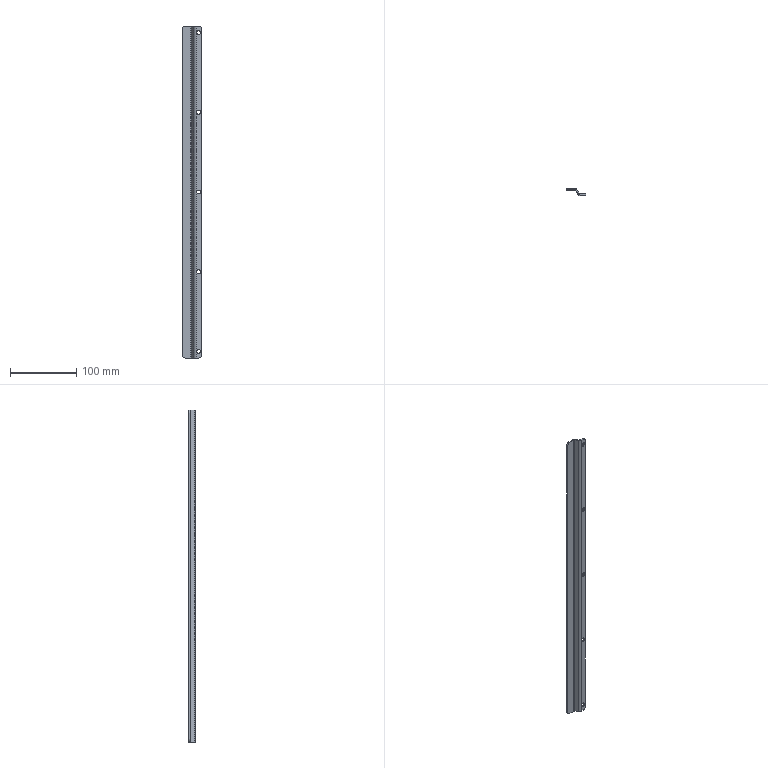Part | NX | features solid 2 | 1 solid | 28 faces | box 30 x 10 x 500 mm | volume 33531 mm3 | cylinder 18 | plane 10 | commonest cylinder face diameters 6 x10 10 x4 4 x2 8 x2
STEP:
#1=CARTESIAN_POINT('',(1918.,-650.,1125.));
#2=VERTEX_POINT('',#1);
#3=CARTESIAN_POINT('',(1918.,-648.,1125.));
#4=VERTEX_POINT('',#3);
#5=CARTESIAN_POINT('',(1918.,-1148.999,1125.));
#6=DIRECTION('',(0.,1.,0.));
#7=VECTOR('',#6,1000.);
#8=LINE('',#5,#7);
#9=EDGE_CURVE('',#2,#4,#8,.T.);
#10=ORIENTED_EDGE('',*,*,#9,.F.);
#11=CARTESIAN_POINT('',(1912.,-650.,1125.));
#12=VERTEX_POINT('',#11);
#13=CARTESIAN_POINT('',(1915.,-650.,1125.));
#14=DIRECTION('',(0.,1.,0.));
#15=DIRECTION('',(-1.,0.,0.));
#16=AXIS2_PLACEMENT_3D('',#13,#14,#15);
#17=CIRCLE('',#16,3.);
#18=EDGE_CURVE('',#12,#2,#17,.T.);
#19=ORIENTED_EDGE('',*,*,#18,.F.);
#20=CARTESIAN_POINT('',(1912.,-648.,1125.));
#21=VERTEX_POINT('',#20);
#22=CARTESIAN_POINT('',(1912.,-1148.999,1125.));
#23=DIRECTION('',(0.,1.,0.));
#24=VECTOR('',#23,1000.);
#25=LINE('',#22,#24);
#26=EDGE_CURVE('',#21,#12,#25,.F.);
#27=ORIENTED_EDGE('',*,*,#26,.F.);
#28=CARTESIAN_POINT('',(1915.,-648.,1125.));
#29=DIRECTION('',(0.,1.,0.));
#30=DIRECTION('',(0.,0.,-1.));
#31=AXIS2_PLACEMENT_3D('',#28,#29,#30);
#32=CIRCLE('',#31,3.);
#33=EDGE_CURVE('',#21,#4,#32,.T.);
#34=ORIENTED_EDGE('',*,*,#33,.T.);
#35=EDGE_LOOP('',(#10,#19,#27,#34));
#36=FACE_BOUND('',#35,.T.);
#37=CARTESIAN_POINT('',(1915.,-1148.999,1125.));
#38=DIRECTION('',(0.,1.,0.));
#39=DIRECTION('',(-1.,0.,0.));
#40=AXIS2_PLACEMENT_3D('',#37,#38,#39);
#41=CYLINDRICAL_SURFACE('',#40,3.);
#42=ADVANCED_FACE('',(#36),#41,.F.);
#43=CARTESIAN_POINT('',(1918.,-650.,645.));
#44=VERTEX_POINT('',#43);
#45=CARTESIAN_POINT('',(1918.,-648.,645.));
#46=VERTEX_POINT('',#45);
#47=CARTESIAN_POINT('',(1918.,-1148.999,645.));
#48=DIRECTION('',(0.,1.,0.));
#49=VECTOR('',#48,1000.);
#50=LINE('',#47,#49);
#51=EDGE_CURVE('',#44,#46,#50,.T.);
#52=ORIENTED_EDGE('',*,*,#51,.F.);
#53=CARTESIAN_POINT('',(1912.,-650.,645.));
#54=VERTEX_POINT('',#53);
#55=CARTESIAN_POINT('',(1915.,-650.,645.));
#56=DIRECTION('',(0.,1.,0.));
#57=DIRECTION('',(-1.,0.,0.));
#58=AXIS2_PLACEMENT_3D('',#55,#56,#57);
#59=CIRCLE('',#58,3.);
#60=EDGE_CURVE('',#54,#44,#59,.T.);
#61=ORIENTED_EDGE('',*,*,#60,.F.);
#62=CARTESIAN_POINT('',(1912.,-648.,645.));
#63=VERTEX_POINT('',#62);
#64=CARTESIAN_POINT('',(1912.,-1148.999,645.));
#65=DIRECTION('',(0.,1.,0.));
#66=VECTOR('',#65,1000.);
#67=LINE('',#64,#66);
#68=EDGE_CURVE('',#63,#54,#67,.F.);
#69=ORIENTED_EDGE('',*,*,#68,.F.);
#70=CARTESIAN_POINT('',(1915.,-648.,645.));
#71=DIRECTION('',(0.,1.,0.));
#72=DIRECTION('',(0.,0.,-1.));
#73=AXIS2_PLACEMENT_3D('',#70,#71,#72);
#74=CIRCLE('',#73,3.);
#75=EDGE_CURVE('',#63,#46,#74,.T.);
#76=ORIENTED_EDGE('',*,*,#75,.T.);
#77=EDGE_LOOP('',(#52,#61,#69,#76));
#78=FACE_BOUND('',#77,.T.);
#79=CARTESIAN_POINT('',(1915.,-1148.999,645.));
#80=DIRECTION('',(0.,1.,0.));
#81=DIRECTION('',(-1.,0.,0.));
#82=AXIS2_PLACEMENT_3D('',#79,#80,#81);
#83=CYLINDRICAL_SURFACE('',#82,3.);
#84=ADVANCED_FACE('',(#78),#83,.F.);
#85=CARTESIAN_POINT('',(1918.,-650.,1005.));
#86=VERTEX_POINT('',#85);
#87=CARTESIAN_POINT('',(1918.,-648.,1005.));
#88=VERTEX_POINT('',#87);
#89=CARTESIAN_POINT('',(1918.,-1148.999,1005.));
#90=DIRECTION('',(0.,1.,0.));
#91=VECTOR('',#90,1000.);
#92=LINE('',#89,#91);
#93=EDGE_CURVE('',#86,#88,#92,.T.);
#94=ORIENTED_EDGE('',*,*,#93,.F.);
#95=CARTESIAN_POINT('',(1912.,-650.,1005.));
#96=VERTEX_POINT('',#95);
#97=CARTESIAN_POINT('',(1915.,-650.,1005.));
#98=DIRECTION('',(0.,1.,0.));
#99=DIRECTION('',(-1.,0.,0.));
#100=AXIS2_PLACEMENT_3D('',#97,#98,#99);
#101=CIRCLE('',#100,3.);
#102=EDGE_CURVE('',#96,#86,#101,.T.);
#103=ORIENTED_EDGE('',*,*,#102,.F.);
#104=CARTESIAN_POINT('',(1912.,-648.,1005.));
#105=VERTEX_POINT('',#104);
#106=CARTESIAN_POINT('',(1912.,-1148.999,1005.));
#107=DIRECTION('',(0.,1.,0.));
#108=VECTOR('',#107,1000.);
#109=LINE('',#106,#108);
#110=EDGE_CURVE('',#105,#96,#109,.F.);
#111=ORIENTED_EDGE('',*,*,#110,.F.);
#112=CARTESIAN_POINT('',(1915.,-648.,1005.));
#113=DIRECTION('',(0.,1.,0.));
#114=DIRECTION('',(0.,0.,-1.));
#115=AXIS2_PLACEMENT_3D('',#112,#113,#114);
#116=CIRCLE('',#115,3.);
#117=EDGE_CURVE('',#105,#88,#116,.T.);
#118=ORIENTED_EDGE('',*,*,#117,.T.);
#119=EDGE_LOOP('',(#94,#103,#111,#118));
#120=FACE_BOUND('',#119,.T.);
#121=CARTESIAN_POINT('',(1915.,-1148.999,1005.));
#122=DIRECTION('',(0.,1.,0.));
#123=DIRECTION('',(-1.,0.,0.));
#124=AXIS2_PLACEMENT_3D('',#121,#122,#123);
#125=CYLINDRICAL_SURFACE('',#124,3.);
#126=ADVANCED_FACE('',(#120),#125,.F.);
#127=CARTESIAN_POINT('',(1918.,-648.,765.));
#128=VERTEX_POINT('',#127);
#129=CARTESIAN_POINT('',(1918.,-650.,765.));
#130=VERTEX_POINT('',#129);
#131=CARTESIAN_POINT('',(1918.,-1148.999,765.));
#132=DIRECTION('',(0.,1.,0.));
#133=VECTOR('',#132,1000.);
#134=LINE('',#131,#133);
#135=EDGE_CURVE('',#128,#130,#134,.F.);
#136=ORIENTED_EDGE('',*,*,#135,.T.);
#137=CARTESIAN_POINT('',(1912.,-650.,765.));
#138=VERTEX_POINT('',#137);
#139=CARTESIAN_POINT('',(1915.,-650.,765.));
#140=DIRECTION('',(0.,1.,0.));
#141=DIRECTION('',(-1.,0.,0.));
#142=AXIS2_PLACEMENT_3D('',#139,#140,#141);
#143=CIRCLE('',#142,3.);
#144=EDGE_CURVE('',#138,#130,#143,.T.);
#145=ORIENTED_EDGE('',*,*,#144,.F.);
#146=CARTESIAN_POINT('',(1912.,-648.,765.));
#147=VERTEX_POINT('',#146);
#148=CARTESIAN_POINT('',(1912.,-1148.999,765.));
#149=DIRECTION('',(0.,1.,0.));
#150=VECTOR('',#149,1000.);
#151=LINE('',#148,#150);
#152=EDGE_CURVE('',#138,#147,#151,.T.);
#153=ORIENTED_EDGE('',*,*,#152,.T.);
#154=CARTESIAN_POINT('',(1915.,-648.,765.));
#155=DIRECTION('',(0.,1.,0.));
#156=DIRECTION('',(0.,0.,-1.));
#157=AXIS2_PLACEMENT_3D('',#154,#155,#156);
#158=CIRCLE('',#157,3.);
#159=EDGE_CURVE('',#147,#128,#158,.T.);
#160=ORIENTED_EDGE('',*,*,#159,.T.);
#161=EDGE_LOOP('',(#136,#145,#153,#160));
#162=FACE_BOUND('',#161,.T.);
#163=CARTESIAN_POINT('',(1915.,-1148.999,765.));
#164=DIRECTION('',(0.,1.,0.));
#165=DIRECTION('',(-1.,0.,0.));
#166=AXIS2_PLACEMENT_3D('',#163,#164,#165);
#167=CYLINDRICAL_SURFACE('',#166,3.);
#168=ADVANCED_FACE('',(#162),#167,.F.);
#169=CARTESIAN_POINT('',(1918.,-650.,885.));
#170=VERTEX_POINT('',#169);
#171=CARTESIAN_POINT('',(1918.,-648.,885.));
#172=VERTEX_POINT('',#171);
#173=CARTESIAN_POINT('',(1918.,-1148.999,885.));
#174=DIRECTION('',(0.,1.,0.));
#175=VECTOR('',#174,1000.);
#176=LINE('',#173,#175);
#177=EDGE_CURVE('',#170,#172,#176,.T.);
#178=ORIENTED_EDGE('',*,*,#177,.F.);
#179=CARTESIAN_POINT('',(1912.,-650.,885.));
#180=VERTEX_POINT('',#179);
#181=CARTESIAN_POINT('',(1915.,-650.,885.));
#182=DIRECTION('',(0.,1.,0.));
#183=DIRECTION('',(-1.,0.,0.));
#184=AXIS2_PLACEMENT_3D('',#181,#182,#183);
#185=CIRCLE('',#184,3.);
#186=EDGE_CURVE('',#180,#170,#185,.T.);
#187=ORIENTED_EDGE('',*,*,#186,.F.);
#188=CARTESIAN_POINT('',(1912.,-648.,885.));
#189=VERTEX_POINT('',#188);
#190=CARTESIAN_POINT('',(1912.,-1148.999,885.));
#191=DIRECTION('',(0.,1.,0.));
#192=VECTOR('',#191,1000.);
#193=LINE('',#190,#192);
#194=EDGE_CURVE('',#189,#180,#193,.F.);
#195=ORIENTED_EDGE('',*,*,#194,.F.);
#196=CARTESIAN_POINT('',(1915.,-648.,885.));
#197=DIRECTION('',(0.,1.,0.));
#198=DIRECTION('',(0.,0.,-1.));
#199=AXIS2_PLACEMENT_3D('',#196,#197,#198);
#200=CIRCLE('',#199,3.);
#201=EDGE_CURVE('',#189,#172,#200,.T.);
#202=ORIENTED_EDGE('',*,*,#201,.T.);
#203=EDGE_LOOP('',(#178,#187,#195,#202));
#204=FACE_BOUND('',#203,.T.);
#205=CARTESIAN_POINT('',(1915.,-1148.999,885.));
#206=DIRECTION('',(0.,1.,0.));
#207=DIRECTION('',(-1.,0.,0.));
#208=AXIS2_PLACEMENT_3D('',#205,#206,#207);
#209=CYLINDRICAL_SURFACE('',#208,3.);
#210=ADVANCED_FACE('',(#204),#209,.F.);
#211=CARTESIAN_POINT('',(1895.,-642.,1135.));
#212=VERTEX_POINT('',#211);
#213=CARTESIAN_POINT('',(1890.,-642.,1130.));
#214=VERTEX_POINT('',#213);
#215=CARTESIAN_POINT('',(1895.,-642.,1130.));
#216=DIRECTION('',(0.,-1.,0.));
#217=DIRECTION('',(0.,0.,1.));
#218=AXIS2_PLACEMENT_3D('',#215,#216,#217);
#219=CIRCLE('',#218,5.);
#220=EDGE_CURVE('',#212,#214,#219,.T.);
#221=ORIENTED_EDGE('',*,*,#220,.F.);
#222=CARTESIAN_POINT('',(1895.,-640.,1135.));
#223=VERTEX_POINT('',#222);
#224=CARTESIAN_POINT('',(1895.,-648.,1135.));
#225=DIRECTION('',(0.,-1.,0.));
#226=VECTOR('',#225,1000.);
#227=LINE('',#224,#226);
#228=EDGE_CURVE('',#223,#212,#227,.T.);
#229=ORIENTED_EDGE('',*,*,#228,.F.);
#230=CARTESIAN_POINT('',(1890.,-640.,1130.));
#231=VERTEX_POINT('',#230);
#232=CARTESIAN_POINT('',(1895.,-640.,1130.));
#233=DIRECTION('',(0.,1.,0.));
#234=DIRECTION('',(0.,0.,1.));
#235=AXIS2_PLACEMENT_3D('',#232,#233,#234);
#236=CIRCLE('',#235,5.);
#237=EDGE_CURVE('',#231,#223,#236,.T.);
#238=ORIENTED_EDGE('',*,*,#237,.F.);
#239=CARTESIAN_POINT('',(1890.,-640.,1130.));
#240=DIRECTION('',(0.,1.,0.));
#241=VECTOR('',#240,1000.);
#242=LINE('',#239,#241);
#243=EDGE_CURVE('',#214,#231,#242,.T.);
#244=ORIENTED_EDGE('',*,*,#243,.F.);
#245=EDGE_LOOP('',(#221,#229,#238,#244));
#246=FACE_BOUND('',#245,.T.);
#247=CARTESIAN_POINT('',(1895.,-640.,1130.));
#248=DIRECTION('',(0.,-1.,0.));
#249=DIRECTION('',(0.,0.,-1.));
#250=AXIS2_PLACEMENT_3D('',#247,#248,#249);
#251=CYLINDRICAL_SURFACE('',#250,5.);
#252=ADVANCED_FACE('',(#246),#251,.T.);
#253=CARTESIAN_POINT('',(1920.,-650.,1130.));
#254=VERTEX_POINT('',#253);
#255=CARTESIAN_POINT('',(1915.,-650.,1135.));
#256=VERTEX_POINT('',#255);
#257=CARTESIAN_POINT('',(1915.,-650.,1130.));
#258=DIRECTION('',(0.,-1.,0.));
#259=DIRECTION('',(-1.,0.,0.));
#260=AXIS2_PLACEMENT_3D('',#257,#258,#259);
#261=CIRCLE('',#260,5.);
#262=EDGE_CURVE('',#254,#256,#261,.T.);
#263=ORIENTED_EDGE('',*,*,#262,.F.);
#264=CARTESIAN_POINT('',(1920.,-648.,1130.));
#265=VERTEX_POINT('',#264);
#266=CARTESIAN_POINT('',(1920.,-648.,1130.));
#267=DIRECTION('',(0.,-1.,0.));
#268=VECTOR('',#267,1000.);
#269=LINE('',#266,#268);
#270=EDGE_CURVE('',#265,#254,#269,.T.);
#271=ORIENTED_EDGE('',*,*,#270,.F.);
#272=CARTESIAN_POINT('',(1915.,-648.,1135.));
#273=VERTEX_POINT('',#272);
#274=CARTESIAN_POINT('',(1915.,-648.,1130.));
#275=DIRECTION('',(0.,1.,0.));
#276=DIRECTION('',(-1.,0.,0.));
#277=AXIS2_PLACEMENT_3D('',#274,#275,#276);
#278=CIRCLE('',#277,5.);
#279=EDGE_CURVE('',#273,#265,#278,.T.);
#280=ORIENTED_EDGE('',*,*,#279,.F.);
#281=CARTESIAN_POINT('',(1915.,-648.,1135.));
#282=DIRECTION('',(0.,1.,0.));
#283=VECTOR('',#282,1000.);
#284=LINE('',#281,#283);
#285=EDGE_CURVE('',#256,#273,#284,.T.);
#286=ORIENTED_EDGE('',*,*,#285,.F.);
#287=EDGE_LOOP('',(#263,#271,#280,#286));
#288=FACE_BOUND('',#287,.T.);
#289=CARTESIAN_POINT('',(1915.,-648.,1130.));
#290=DIRECTION('',(0.,1.,0.));
#291=DIRECTION('',(-1.,0.,0.));
#292=AXIS2_PLACEMENT_3D('',#289,#290,#291);
#293=CYLINDRICAL_SURFACE('',#292,5.);
#294=ADVANCED_FACE('',(#288),#293,.T.);
#295=CARTESIAN_POINT('',(1890.,-642.,640.));
#296=VERTEX_POINT('',#295);
#297=CARTESIAN_POINT('',(1895.,-642.,635.));
#298=VERTEX_POINT('',#297);
#299=CARTESIAN_POINT('',(1895.,-642.,640.));
#300=DIRECTION('',(0.,-1.,0.));
#301=DIRECTION('',(0.,0.,1.));
#302=AXIS2_PLACEMENT_3D('',#299,#300,#301);
#303=CIRCLE('',#302,5.);
#304=EDGE_CURVE('',#296,#298,#303,.T.);
#305=ORIENTED_EDGE('',*,*,#304,.F.);
#306=CARTESIAN_POINT('',(1890.,-640.,640.));
#307=VERTEX_POINT('',#306);
#308=CARTESIAN_POINT('',(1890.,-640.,640.));
#309=DIRECTION('',(0.,-1.,0.));
#310=VECTOR('',#309,1000.);
#311=LINE('',#308,#310);
#312=EDGE_CURVE('',#307,#296,#311,.T.);
#313=ORIENTED_EDGE('',*,*,#312,.F.);
#314=CARTESIAN_POINT('',(1895.,-640.,635.));
#315=VERTEX_POINT('',#314);
#316=CARTESIAN_POINT('',(1895.,-640.,640.));
#317=DIRECTION('',(0.,1.,0.));
#318=DIRECTION('',(0.,0.,1.));
#319=AXIS2_PLACEMENT_3D('',#316,#317,#318);
#320=CIRCLE('',#319,5.);
#321=EDGE_CURVE('',#315,#307,#320,.T.);
#322=ORIENTED_EDGE('',*,*,#321,.F.);
#323=CARTESIAN_POINT('',(1895.,-640.,635.));
#324=DIRECTION('',(0.,1.,0.));
#325=VECTOR('',#324,1000.);
#326=LINE('',#323,#325);
#327=EDGE_CURVE('',#298,#315,#326,.T.);
#328=ORIENTED_EDGE('',*,*,#327,.F.);
#329=EDGE_LOOP('',(#305,#313,#322,#328));
#330=FACE_BOUND('',#329,.T.);
#331=CARTESIAN_POINT('',(1895.,-640.,640.));
#332=DIRECTION('',(0.,1.,0.));
#333=DIRECTION('',(0.,0.,1.));
#334=AXIS2_PLACEMENT_3D('',#331,#332,#333);
#335=CYLINDRICAL_SURFACE('',#334,5.);
#336=ADVANCED_FACE('',(#330),#335,.T.);
#337=CARTESIAN_POINT('',(1915.,-650.,635.));
#338=VERTEX_POINT('',#337);
#339=CARTESIAN_POINT('',(1920.,-650.,640.));
#340=VERTEX_POINT('',#339);
#341=CARTESIAN_POINT('',(1915.,-650.,640.));
#342=DIRECTION('',(0.,-1.,0.));
#343=DIRECTION('',(-1.,0.,0.));
#344=AXIS2_PLACEMENT_3D('',#341,#342,#343);
#345=CIRCLE('',#344,5.);
#346=EDGE_CURVE('',#338,#340,#345,.T.);
#347=ORIENTED_EDGE('',*,*,#346,.F.);
#348=CARTESIAN_POINT('',(1915.,-648.,635.));
#349=VERTEX_POINT('',#348);
#350=CARTESIAN_POINT('',(1915.,-640.,635.));
#351=DIRECTION('',(0.,-1.,0.));
#352=VECTOR('',#351,1000.);
#353=LINE('',#350,#352);
#354=EDGE_CURVE('',#349,#338,#353,.T.);
#355=ORIENTED_EDGE('',*,*,#354,.F.);
#356=CARTESIAN_POINT('',(1920.,-648.,640.));
#357=VERTEX_POINT('',#356);
#358=CARTESIAN_POINT('',(1915.,-648.,640.));
#359=DIRECTION('',(0.,1.,0.));
#360=DIRECTION('',(-1.,0.,0.));
#361=AXIS2_PLACEMENT_3D('',#358,#359,#360);
#362=CIRCLE('',#361,5.);
#363=EDGE_CURVE('',#357,#349,#362,.T.);
#364=ORIENTED_EDGE('',*,*,#363,.F.);
#365=CARTESIAN_POINT('',(1920.,-648.,640.));
#366=DIRECTION('',(0.,1.,0.));
#367=VECTOR('',#366,1000.);
#368=LINE('',#365,#367);
#369=EDGE_CURVE('',#340,#357,#368,.T.);
#370=ORIENTED_EDGE('',*,*,#369,.F.);
#371=EDGE_LOOP('',(#347,#355,#364,#370));
#372=FACE_BOUND('',#371,.T.);
#373=CARTESIAN_POINT('',(1915.,-648.,640.));
#374=DIRECTION('',(0.,-1.,0.));
#375=DIRECTION('',(1.,0.,0.));
#376=AXIS2_PLACEMENT_3D('',#373,#374,#375);
#377=CYLINDRICAL_SURFACE('',#376,5.);
#378=ADVANCED_FACE('',(#372),#377,.T.);
#379=CARTESIAN_POINT('',(1890.,-642.,635.));
#380=DIRECTION('',(0.,0.,1.));
#381=VECTOR('',#380,1000.);
#382=LINE('',#379,#381);
#383=EDGE_CURVE('',#296,#214,#382,.T.);
#384=ORIENTED_EDGE('',*,*,#383,.F.);
#385=ORIENTED_EDGE('',*,*,#304,.T.);
#386=CARTESIAN_POINT('',(1902.783,-642.,635.));
#387=VERTEX_POINT('',#386);
#388=CARTESIAN_POINT('',(1905.,-642.,635.));
#389=DIRECTION('',(-1.,0.,0.));
#390=VECTOR('',#389,1000.);
#391=LINE('',#388,#390);
#392=EDGE_CURVE('',#387,#298,#391,.T.);
#393=ORIENTED_EDGE('',*,*,#392,.F.);
#394=CARTESIAN_POINT('',(1902.783,-642.,1135.));
#395=VERTEX_POINT('',#394);
#396=CARTESIAN_POINT('',(1902.783,-642.,635.));
#397=DIRECTION('',(0.,0.,1.));
#398=VECTOR('',#397,1000.);
#399=LINE('',#396,#398);
#400=EDGE_CURVE('',#387,#395,#399,.T.);
#401=ORIENTED_EDGE('',*,*,#400,.T.);
#402=CARTESIAN_POINT('',(1905.,-642.,1135.));
#403=DIRECTION('',(-1.,0.,0.));
#404=VECTOR('',#403,1000.);
#405=LINE('',#402,#404);
#406=EDGE_CURVE('',#395,#212,#405,.T.);
#407=ORIENTED_EDGE('',*,*,#406,.T.);
#408=ORIENTED_EDGE('',*,*,#220,.T.);
#409=EDGE_LOOP('',(#384,#385,#393,#401,#407,#408));
#410=FACE_BOUND('',#409,.T.);
#411=CARTESIAN_POINT('',(1905.,-642.,635.));
#412=DIRECTION('',(0.,1.,0.));
#413=DIRECTION('',(0.,0.,-1.));
#414=AXIS2_PLACEMENT_3D('',#411,#412,#413);
#415=PLANE('',#414);
#416=ADVANCED_FACE('',(#410),#415,.F.);
#417=CARTESIAN_POINT('',(1904.479,-642.94,1135.));
#418=VERTEX_POINT('',#417);
#419=CARTESIAN_POINT('',(1902.783,-644.,1135.));
#420=DIRECTION('',(0.,0.,1.));
#421=DIRECTION('',(0.,-1.,0.));
#422=AXIS2_PLACEMENT_3D('',#419,#420,#421);
#423=CIRCLE('',#422,2.);
#424=EDGE_CURVE('',#418,#395,#423,.T.);
#425=ORIENTED_EDGE('',*,*,#424,.T.);
#426=ORIENTED_EDGE('',*,*,#400,.F.);
#427=CARTESIAN_POINT('',(1904.479,-642.94,635.));
#428=VERTEX_POINT('',#427);
#429=CARTESIAN_POINT('',(1902.783,-644.,635.));
#430=DIRECTION('',(0.,0.,1.));
#431=DIRECTION('',(0.,-1.,0.));
#432=AXIS2_PLACEMENT_3D('',#429,#430,#431);
#433=CIRCLE('',#432,2.);
#434=EDGE_CURVE('',#428,#387,#433,.T.);
#435=ORIENTED_EDGE('',*,*,#434,.F.);
#436=CARTESIAN_POINT('',(1904.479,-642.94,635.));
#437=DIRECTION('',(0.,0.,1.));
#438=VECTOR('',#437,1000.);
#439=LINE('',#436,#438);
#440=EDGE_CURVE('',#428,#418,#439,.T.);
#441=ORIENTED_EDGE('',*,*,#440,.T.);
#442=EDGE_LOOP('',(#425,#426,#435,#441));
#443=FACE_BOUND('',#442,.T.);
#444=CARTESIAN_POINT('',(1902.783,-644.,635.));
#445=DIRECTION('',(0.,0.,1.));
#446=DIRECTION('',(0.,-1.,0.));
#447=AXIS2_PLACEMENT_3D('',#444,#445,#446);
#448=CYLINDRICAL_SURFACE('',#447,2.);
#449=ADVANCED_FACE('',(#443),#448,.F.);
#450=CARTESIAN_POINT('',(1907.717,-648.12,1135.));
#451=VERTEX_POINT('',#450);
#452=CARTESIAN_POINT('',(1908.304,-649.06,1135.));
#453=DIRECTION('',(-0.53,0.848,0.));
#454=VECTOR('',#453,1000.);
#455=LINE('',#452,#454);
#456=EDGE_CURVE('',#451,#418,#455,.T.);
#457=ORIENTED_EDGE('',*,*,#456,.T.);
#458=ORIENTED_EDGE('',*,*,#440,.F.);
#459=CARTESIAN_POINT('',(1907.717,-648.12,635.));
#460=VERTEX_POINT('',#459);
#461=CARTESIAN_POINT('',(1908.304,-649.06,635.));
#462=DIRECTION('',(-0.53,0.848,0.));
#463=VECTOR('',#462,1000.);
#464=LINE('',#461,#463);
#465=EDGE_CURVE('',#460,#428,#464,.T.);
#466=ORIENTED_EDGE('',*,*,#465,.F.);
#467=CARTESIAN_POINT('',(1907.717,-648.12,635.));
#468=DIRECTION('',(0.,0.,1.));
#469=VECTOR('',#468,1000.);
#470=LINE('',#467,#469);
#471=EDGE_CURVE('',#460,#451,#470,.T.);
#472=ORIENTED_EDGE('',*,*,#471,.T.);
#473=EDGE_LOOP('',(#457,#458,#466,#472));
#474=FACE_BOUND('',#473,.T.);
#475=CARTESIAN_POINT('',(1908.304,-649.06,635.));
#476=DIRECTION('',(0.848,0.53,0.));
#477=DIRECTION('',(0.,0.,-1.));
#478=AXIS2_PLACEMENT_3D('',#475,#476,#477);
#479=PLANE('',#478);
#480=ADVANCED_FACE('',(#474),#479,.F.);
#481=CARTESIAN_POINT('',(1911.108,-650.,1135.));
#482=VERTEX_POINT('',#481);
#483=CARTESIAN_POINT('',(1911.108,-646.,1135.));
#484=DIRECTION('',(0.,0.,-1.));
#485=DIRECTION('',(0.,-1.,0.));
#486=AXIS2_PLACEMENT_3D('',#483,#484,#485);
#487=CIRCLE('',#486,4.);
#488=EDGE_CURVE('',#482,#451,#487,.T.);
#489=ORIENTED_EDGE('',*,*,#488,.T.);
#490=ORIENTED_EDGE('',*,*,#471,.F.);
#491=CARTESIAN_POINT('',(1911.108,-650.,635.));
#492=VERTEX_POINT('',#491);
#493=CARTESIAN_POINT('',(1911.108,-646.,635.));
#494=DIRECTION('',(0.,0.,-1.));
#495=DIRECTION('',(0.,-1.,0.));
#496=AXIS2_PLACEMENT_3D('',#493,#494,#495);
#497=CIRCLE('',#496,4.);
#498=EDGE_CURVE('',#492,#460,#497,.T.);
#499=ORIENTED_EDGE('',*,*,#498,.F.);
#500=CARTESIAN_POINT('',(1911.108,-650.,635.));
#501=DIRECTION('',(0.,0.,1.));
#502=VECTOR('',#501,1000.);
#503=LINE('',#500,#502);
#504=EDGE_CURVE('',#492,#482,#503,.T.);
#505=ORIENTED_EDGE('',*,*,#504,.T.);
#506=EDGE_LOOP('',(#489,#490,#499,#505));
#507=FACE_BOUND('',#506,.T.);
#508=CARTESIAN_POINT('',(1911.108,-646.,635.));
#509=DIRECTION('',(0.,0.,1.));
#510=DIRECTION('',(0.,-1.,0.));
#511=AXIS2_PLACEMENT_3D('',#508,#509,#510);
#512=CYLINDRICAL_SURFACE('',#511,4.);
#513=ADVANCED_FACE('',(#507),#512,.T.);
#514=ORIENTED_EDGE('',*,*,#186,.T.);
#515=CARTESIAN_POINT('',(1915.,-650.,885.));
#516=DIRECTION('',(0.,1.,0.));
#517=DIRECTION('',(-1.,0.,0.));
#518=AXIS2_PLACEMENT_3D('',#515,#516,#517);
#519=CIRCLE('',#518,3.);
#520=EDGE_CURVE('',#170,#180,#519,.T.);
#521=ORIENTED_EDGE('',*,*,#520,.T.);
#522=EDGE_LOOP('',(#514,#521));
#523=FACE_BOUND('',#522,.T.);
#524=ORIENTED_EDGE('',*,*,#144,.T.);
#525=CARTESIAN_POINT('',(1915.,-650.,765.));
#526=DIRECTION('',(0.,1.,0.));
#527=DIRECTION('',(-1.,0.,0.));
#528=AXIS2_PLACEMENT_3D('',#525,#526,#527);
#529=CIRCLE('',#528,3.);
#530=EDGE_CURVE('',#130,#138,#529,.T.);
#531=ORIENTED_EDGE('',*,*,#530,.T.);
#532=EDGE_LOOP('',(#524,#531));
#533=FACE_BOUND('',#532,.T.);
#534=ORIENTED_EDGE('',*,*,#102,.T.);
#535=CARTESIAN_POINT('',(1915.,-650.,1005.));
#536=DIRECTION('',(0.,1.,0.));
#537=DIRECTION('',(-1.,0.,0.));
#538=AXIS2_PLACEMENT_3D('',#535,#536,#537);
#539=CIRCLE('',#538,3.);
#540=EDGE_CURVE('',#86,#96,#539,.T.);
#541=ORIENTED_EDGE('',*,*,#540,.T.);
#542=EDGE_LOOP('',(#534,#541));
#543=FACE_BOUND('',#542,.T.);
#544=ORIENTED_EDGE('',*,*,#60,.T.);
#545=CARTESIAN_POINT('',(1915.,-650.,645.));
#546=DIRECTION('',(0.,1.,0.));
#547=DIRECTION('',(-1.,0.,0.));
#548=AXIS2_PLACEMENT_3D('',#545,#546,#547);
#549=CIRCLE('',#548,3.);
#550=EDGE_CURVE('',#44,#54,#549,.T.);
#551=ORIENTED_EDGE('',*,*,#550,.T.);
#552=EDGE_LOOP('',(#544,#551));
#553=FACE_BOUND('',#552,.T.);
#554=ORIENTED_EDGE('',*,*,#18,.T.);
#555=CARTESIAN_POINT('',(1915.,-650.,1125.));
#556=DIRECTION('',(0.,1.,0.));
#557=DIRECTION('',(-1.,0.,0.));
#558=AXIS2_PLACEMENT_3D('',#555,#556,#557);
#559=CIRCLE('',#558,3.);
#560=EDGE_CURVE('',#2,#12,#559,.T.);
#561=ORIENTED_EDGE('',*,*,#560,.T.);
#562=EDGE_LOOP('',(#554,#561));
#563=FACE_BOUND('',#562,.T.);
#564=CARTESIAN_POINT('',(1920.,-650.,635.));
#565=DIRECTION('',(-1.,0.,0.));
#566=VECTOR('',#565,1000.);
#567=LINE('',#564,#566);
#568=EDGE_CURVE('',#338,#492,#567,.T.);
#569=ORIENTED_EDGE('',*,*,#568,.F.);
#570=ORIENTED_EDGE('',*,*,#346,.T.);
#571=CARTESIAN_POINT('',(1920.,-650.,635.));
#572=DIRECTION('',(0.,0.,1.));
#573=VECTOR('',#572,1000.);
#574=LINE('',#571,#573);
#575=EDGE_CURVE('',#340,#254,#574,.T.);
#576=ORIENTED_EDGE('',*,*,#575,.T.);
#577=ORIENTED_EDGE('',*,*,#262,.T.);
#578=CARTESIAN_POINT('',(1920.,-650.,1135.));
#579=DIRECTION('',(-1.,0.,0.));
#580=VECTOR('',#579,1000.);
#581=LINE('',#578,#580);
#582=EDGE_CURVE('',#256,#482,#581,.T.);
#583=ORIENTED_EDGE('',*,*,#582,.T.);
#584=ORIENTED_EDGE('',*,*,#504,.F.);
#585=EDGE_LOOP('',(#569,#570,#576,#577,#583,#584));
#586=FACE_BOUND('',#585,.T.);
#587=CARTESIAN_POINT('',(1920.,-650.,635.));
#588=DIRECTION('',(0.,1.,0.));
#589=DIRECTION('',(0.,0.,-1.));
#590=AXIS2_PLACEMENT_3D('',#587,#588,#589);
#591=PLANE('',#590);
#592=ADVANCED_FACE('',(#523,#533,#543,#553,#563,#586),#591,.F.);
#593=CARTESIAN_POINT('',(1902.783,-640.,635.));
#594=VERTEX_POINT('',#593);
#595=CARTESIAN_POINT('',(1905.,-640.,635.));
#596=DIRECTION('',(-1.,0.,0.));
#597=VECTOR('',#596,1000.);
#598=LINE('',#595,#597);
#599=EDGE_CURVE('',#594,#315,#598,.T.);
#600=ORIENTED_EDGE('',*,*,#599,.T.);
#601=ORIENTED_EDGE('',*,*,#321,.T.);
#602=CARTESIAN_POINT('',(1890.,-640.,635.));
#603=DIRECTION('',(0.,0.,1.));
#604=VECTOR('',#603,1000.);
#605=LINE('',#602,#604);
#606=EDGE_CURVE('',#307,#231,#605,.T.);
#607=ORIENTED_EDGE('',*,*,#606,.T.);
#608=ORIENTED_EDGE('',*,*,#237,.T.);
#609=CARTESIAN_POINT('',(1902.783,-640.,1135.));
#610=VERTEX_POINT('',#609);
#611=CARTESIAN_POINT('',(1905.,-640.,1135.));
#612=DIRECTION('',(-1.,0.,0.));
#613=VECTOR('',#612,1000.);
#614=LINE('',#611,#613);
#615=EDGE_CURVE('',#610,#223,#614,.T.);
#616=ORIENTED_EDGE('',*,*,#615,.F.);
#617=CARTESIAN_POINT('',(1902.783,-640.,635.));
#618=DIRECTION('',(0.,0.,1.));
#619=VECTOR('',#618,1000.);
#620=LINE('',#617,#619);
#621=EDGE_CURVE('',#594,#610,#620,.T.);
#622=ORIENTED_EDGE('',*,*,#621,.F.);
#623=EDGE_LOOP('',(#600,#601,#607,#608,#616,#622));
#624=FACE_BOUND('',#623,.T.);
#625=CARTESIAN_POINT('',(1905.,-640.,635.));
#626=DIRECTION('',(0.,1.,0.));
#627=DIRECTION('',(0.,0.,-1.));
#628=AXIS2_PLACEMENT_3D('',#625,#626,#627);
#629=PLANE('',#628);
#630=ADVANCED_FACE('',(#624),#629,.T.);
#631=CARTESIAN_POINT('',(1906.175,-641.88,1135.));
#632=VERTEX_POINT('',#631);
#633=CARTESIAN_POINT('',(1902.783,-644.,1135.));
#634=DIRECTION('',(0.,0.,1.));
#635=DIRECTION('',(0.,1.,0.));
#636=AXIS2_PLACEMENT_3D('',#633,#634,#635);
#637=CIRCLE('',#636,4.);
#638=EDGE_CURVE('',#632,#610,#637,.T.);
#639=ORIENTED_EDGE('',*,*,#638,.F.);
#640=CARTESIAN_POINT('',(1906.175,-641.88,635.));
#641=VERTEX_POINT('',#640);
#642=CARTESIAN_POINT('',(1906.175,-641.88,635.));
#643=DIRECTION('',(0.,0.,1.));
#644=VECTOR('',#643,1000.);
#645=LINE('',#642,#644);
#646=EDGE_CURVE('',#641,#632,#645,.T.);
#647=ORIENTED_EDGE('',*,*,#646,.F.);
#648=CARTESIAN_POINT('',(1902.783,-644.,635.));
#649=DIRECTION('',(0.,0.,1.));
#650=DIRECTION('',(0.,1.,0.));
#651=AXIS2_PLACEMENT_3D('',#648,#649,#650);
#652=CIRCLE('',#651,4.);
#653=EDGE_CURVE('',#641,#594,#652,.T.);
#654=ORIENTED_EDGE('',*,*,#653,.T.);
#655=ORIENTED_EDGE('',*,*,#621,.T.);
#656=EDGE_LOOP('',(#639,#647,#654,#655));
#657=FACE_BOUND('',#656,.T.);
#658=CARTESIAN_POINT('',(1902.783,-644.,635.));
#659=DIRECTION('',(0.,0.,1.));
#660=DIRECTION('',(0.,-1.,0.));
#661=AXIS2_PLACEMENT_3D('',#658,#659,#660);
#662=CYLINDRICAL_SURFACE('',#661,4.);
#663=ADVANCED_FACE('',(#657),#662,.T.);
#664=CARTESIAN_POINT('',(1909.412,-647.06,1135.));
#665=VERTEX_POINT('',#664);
#666=CARTESIAN_POINT('',(1910.,-648.,1135.));
#667=DIRECTION('',(-0.53,0.848,0.));
#668=VECTOR('',#667,1000.);
#669=LINE('',#666,#668);
#670=EDGE_CURVE('',#665,#632,#669,.T.);
#671=ORIENTED_EDGE('',*,*,#670,.F.);
#672=CARTESIAN_POINT('',(1909.412,-647.06,635.));
#673=VERTEX_POINT('',#672);
#674=CARTESIAN_POINT('',(1909.412,-647.06,635.));
#675=DIRECTION('',(0.,0.,1.));
#676=VECTOR('',#675,1000.);
#677=LINE('',#674,#676);
#678=EDGE_CURVE('',#673,#665,#677,.T.);
#679=ORIENTED_EDGE('',*,*,#678,.F.);
#680=CARTESIAN_POINT('',(1910.,-648.,635.));
#681=DIRECTION('',(-0.53,0.848,0.));
#682=VECTOR('',#681,1000.);
#683=LINE('',#680,#682);
#684=EDGE_CURVE('',#673,#641,#683,.T.);
#685=ORIENTED_EDGE('',*,*,#684,.T.);
#686=ORIENTED_EDGE('',*,*,#646,.T.);
#687=EDGE_LOOP('',(#671,#679,#685,#686));
#688=FACE_BOUND('',#687,.T.);
#689=CARTESIAN_POINT('',(1910.,-648.,635.));
#690=DIRECTION('',(0.848,0.53,0.));
#691=DIRECTION('',(0.,0.,-1.));
#692=AXIS2_PLACEMENT_3D('',#689,#690,#691);
#693=PLANE('',#692);
#694=ADVANCED_FACE('',(#688),#693,.T.);
#695=CARTESIAN_POINT('',(1911.108,-648.,1135.));
#696=VERTEX_POINT('',#695);
#697=CARTESIAN_POINT('',(1911.108,-646.,1135.));
#698=DIRECTION('',(0.,0.,-1.));
#699=DIRECTION('',(0.,-1.,0.));
#700=AXIS2_PLACEMENT_3D('',#697,#698,#699);
#701=CIRCLE('',#700,2.);
#702=EDGE_CURVE('',#696,#665,#701,.T.);
#703=ORIENTED_EDGE('',*,*,#702,.F.);
#704=CARTESIAN_POINT('',(1911.108,-648.,635.));
#705=VERTEX_POINT('',#704);
#706=CARTESIAN_POINT('',(1911.108,-648.,635.));
#707=DIRECTION('',(0.,0.,1.));
#708=VECTOR('',#707,1000.);
#709=LINE('',#706,#708);
#710=EDGE_CURVE('',#705,#696,#709,.T.);
#711=ORIENTED_EDGE('',*,*,#710,.F.);
#712=CARTESIAN_POINT('',(1911.108,-646.,635.));
#713=DIRECTION('',(0.,0.,-1.));
#714=DIRECTION('',(0.,-1.,0.));
#715=AXIS2_PLACEMENT_3D('',#712,#713,#714);
#716=CIRCLE('',#715,2.);
#717=EDGE_CURVE('',#705,#673,#716,.T.);
#718=ORIENTED_EDGE('',*,*,#717,.T.);
#719=ORIENTED_EDGE('',*,*,#678,.T.);
#720=EDGE_LOOP('',(#703,#711,#718,#719));
#721=FACE_BOUND('',#720,.T.);
#722=CARTESIAN_POINT('',(1911.108,-646.,635.));
#723=DIRECTION('',(0.,0.,1.));
#724=DIRECTION('',(0.,-1.,0.));
#725=AXIS2_PLACEMENT_3D('',#722,#723,#724);
#726=CYLINDRICAL_SURFACE('',#725,2.);
#727=ADVANCED_FACE('',(#721),#726,.F.);
#728=ORIENTED_EDGE('',*,*,#201,.F.);
#729=CARTESIAN_POINT('',(1915.,-648.,885.));
#730=DIRECTION('',(0.,1.,0.));
#731=DIRECTION('',(0.,0.,-1.));
#732=AXIS2_PLACEMENT_3D('',#729,#730,#731);
#733=CIRCLE('',#732,3.);
#734=EDGE_CURVE('',#172,#189,#733,.T.);
#735=ORIENTED_EDGE('',*,*,#734,.F.);
#736=EDGE_LOOP('',(#728,#735));
#737=FACE_BOUND('',#736,.T.);
#738=ORIENTED_EDGE('',*,*,#159,.F.);
#739=CARTESIAN_POINT('',(1915.,-648.,765.));
#740=DIRECTION('',(0.,1.,0.));
#741=DIRECTION('',(0.,0.,-1.));
#742=AXIS2_PLACEMENT_3D('',#739,#740,#741);
#743=CIRCLE('',#742,3.);
#744=EDGE_CURVE('',#128,#147,#743,.T.);
#745=ORIENTED_EDGE('',*,*,#744,.F.);
#746=EDGE_LOOP('',(#738,#745));
#747=FACE_BOUND('',#746,.T.);
#748=ORIENTED_EDGE('',*,*,#117,.F.);
#749=CARTESIAN_POINT('',(1915.,-648.,1005.));
#750=DIRECTION('',(0.,1.,0.));
#751=DIRECTION('',(0.,0.,-1.));
#752=AXIS2_PLACEMENT_3D('',#749,#750,#751);
#753=CIRCLE('',#752,3.);
#754=EDGE_CURVE('',#88,#105,#753,.T.);
#755=ORIENTED_EDGE('',*,*,#754,.F.);
#756=EDGE_LOOP('',(#748,#755));
#757=FACE_BOUND('',#756,.T.);
#758=ORIENTED_EDGE('',*,*,#75,.F.);
#759=CARTESIAN_POINT('',(1915.,-648.,645.));
#760=DIRECTION('',(0.,1.,0.));
#761=DIRECTION('',(0.,0.,-1.));
#762=AXIS2_PLACEMENT_3D('',#759,#760,#761);
#763=CIRCLE('',#762,3.);
#764=EDGE_CURVE('',#46,#63,#763,.T.);
#765=ORIENTED_EDGE('',*,*,#764,.F.);
#766=EDGE_LOOP('',(#758,#765));
#767=FACE_BOUND('',#766,.T.);
#768=ORIENTED_EDGE('',*,*,#33,.F.);
#769=CARTESIAN_POINT('',(1915.,-648.,1125.));
#770=DIRECTION('',(0.,1.,0.));
#771=DIRECTION('',(0.,0.,-1.));
#772=AXIS2_PLACEMENT_3D('',#769,#770,#771);
#773=CIRCLE('',#772,3.);
#774=EDGE_CURVE('',#4,#21,#773,.T.);
#775=ORIENTED_EDGE('',*,*,#774,.F.);
#776=EDGE_LOOP('',(#768,#775));
#777=FACE_BOUND('',#776,.T.);
#778=CARTESIAN_POINT('',(1920.,-648.,635.));
#779=DIRECTION('',(0.,0.,1.));
#780=VECTOR('',#779,1000.);
#781=LINE('',#778,#780);
#782=EDGE_CURVE('',#357,#265,#781,.T.);
#783=ORIENTED_EDGE('',*,*,#782,.F.);
#784=ORIENTED_EDGE('',*,*,#363,.T.);
#785=CARTESIAN_POINT('',(1920.,-648.,635.));
#786=DIRECTION('',(-1.,0.,0.));
#787=VECTOR('',#786,1000.);
#788=LINE('',#785,#787);
#789=EDGE_CURVE('',#349,#705,#788,.T.);
#790=ORIENTED_EDGE('',*,*,#789,.T.);
#791=ORIENTED_EDGE('',*,*,#710,.T.);
#792=CARTESIAN_POINT('',(1920.,-648.,1135.));
#793=DIRECTION('',(-1.,0.,0.));
#794=VECTOR('',#793,1000.);
#795=LINE('',#792,#794);
#796=EDGE_CURVE('',#273,#696,#795,.T.);
#797=ORIENTED_EDGE('',*,*,#796,.F.);
#798=ORIENTED_EDGE('',*,*,#279,.T.);
#799=EDGE_LOOP('',(#783,#784,#790,#791,#797,#798));
#800=FACE_BOUND('',#799,.T.);
#801=CARTESIAN_POINT('',(1920.,-648.,635.));
#802=DIRECTION('',(0.,1.,0.));
#803=DIRECTION('',(0.,0.,-1.));
#804=AXIS2_PLACEMENT_3D('',#801,#802,#803);
#805=PLANE('',#804);
#806=ADVANCED_FACE('',(#737,#747,#757,#767,#777,#800),#805,.T.);
#807=ORIENTED_EDGE('',*,*,#575,.F.);
#808=ORIENTED_EDGE('',*,*,#369,.T.);
#809=ORIENTED_EDGE('',*,*,#782,.T.);
#810=ORIENTED_EDGE('',*,*,#270,.T.);
#811=EDGE_LOOP('',(#807,#808,#809,#810));
#812=FACE_BOUND('',#811,.T.);
#813=CARTESIAN_POINT('',(1920.,-648.,635.));
#814=DIRECTION('',(-1.,0.,0.));
#815=DIRECTION('',(0.,0.,1.));
#816=AXIS2_PLACEMENT_3D('',#813,#814,#815);
#817=PLANE('',#816);
#818=ADVANCED_FACE('',(#812),#817,.F.);
#819=ORIENTED_EDGE('',*,*,#582,.F.);
#820=ORIENTED_EDGE('',*,*,#285,.T.);
#821=ORIENTED_EDGE('',*,*,#796,.T.);
#822=ORIENTED_EDGE('',*,*,#702,.T.);
#823=ORIENTED_EDGE('',*,*,#670,.T.);
#824=ORIENTED_EDGE('',*,*,#638,.T.);
#825=ORIENTED_EDGE('',*,*,#615,.T.);
#826=ORIENTED_EDGE('',*,*,#228,.T.);
#827=ORIENTED_EDGE('',*,*,#406,.F.);
#828=ORIENTED_EDGE('',*,*,#424,.F.);
#829=ORIENTED_EDGE('',*,*,#456,.F.);
#830=ORIENTED_EDGE('',*,*,#488,.F.);
#831=EDGE_LOOP('',(#819,#820,#821,#822,#823,#824,#825,#826,#827,#828,#829,#830));
#832=FACE_BOUND('',#831,.T.);
#833=CARTESIAN_POINT('',(1920.,-648.,1135.));
#834=DIRECTION('',(0.,0.,-1.));
#835=DIRECTION('',(0.,-1.,0.));
#836=AXIS2_PLACEMENT_3D('',#833,#834,#835);
#837=PLANE('',#836);
#838=ADVANCED_FACE('',(#832),#837,.F.);
#839=ORIENTED_EDGE('',*,*,#606,.F.);
#840=ORIENTED_EDGE('',*,*,#312,.T.);
#841=ORIENTED_EDGE('',*,*,#383,.T.);
#842=ORIENTED_EDGE('',*,*,#243,.T.);
#843=EDGE_LOOP('',(#839,#840,#841,#842));
#844=FACE_BOUND('',#843,.T.);
#845=CARTESIAN_POINT('',(1890.,-640.,635.));
#846=DIRECTION('',(-1.,0.,0.));
#847=DIRECTION('',(0.,0.,1.));
#848=AXIS2_PLACEMENT_3D('',#845,#846,#847);
#849=PLANE('',#848);
#850=ADVANCED_FACE('',(#844),#849,.T.);
#851=ORIENTED_EDGE('',*,*,#789,.F.);
#852=ORIENTED_EDGE('',*,*,#354,.T.);
#853=ORIENTED_EDGE('',*,*,#568,.T.);
#854=ORIENTED_EDGE('',*,*,#498,.T.);
#855=ORIENTED_EDGE('',*,*,#465,.T.);
#856=ORIENTED_EDGE('',*,*,#434,.T.);
#857=ORIENTED_EDGE('',*,*,#392,.T.);
#858=ORIENTED_EDGE('',*,*,#327,.T.);
#859=ORIENTED_EDGE('',*,*,#599,.F.);
#860=ORIENTED_EDGE('',*,*,#653,.F.);
#861=ORIENTED_EDGE('',*,*,#684,.F.);
#862=ORIENTED_EDGE('',*,*,#717,.F.);
#863=EDGE_LOOP('',(#851,#852,#853,#854,#855,#856,#857,#858,#859,#860,#861,#862));
#864=FACE_BOUND('',#863,.T.);
#865=CARTESIAN_POINT('',(1905.,-640.,635.));
#866=DIRECTION('',(0.,0.,-1.));
#867=DIRECTION('',(0.,-1.,0.));
#868=AXIS2_PLACEMENT_3D('',#865,#866,#867);
#869=PLANE('',#868);
#870=ADVANCED_FACE('',(#864),#869,.T.);
#871=ORIENTED_EDGE('',*,*,#520,.F.);
#872=ORIENTED_EDGE('',*,*,#177,.T.);
#873=ORIENTED_EDGE('',*,*,#734,.T.);
#874=ORIENTED_EDGE('',*,*,#194,.T.);
#875=EDGE_LOOP('',(#871,#872,#873,#874));
#876=FACE_BOUND('',#875,.T.);
#877=CARTESIAN_POINT('',(1915.,-1148.999,885.));
#878=DIRECTION('',(0.,1.,0.));
#879=DIRECTION('',(-1.,0.,0.));
#880=AXIS2_PLACEMENT_3D('',#877,#878,#879);
#881=CYLINDRICAL_SURFACE('',#880,3.);
#882=ADVANCED_FACE('',(#876),#881,.F.);
#883=ORIENTED_EDGE('',*,*,#530,.F.);
#884=ORIENTED_EDGE('',*,*,#135,.F.);
#885=ORIENTED_EDGE('',*,*,#744,.T.);
#886=ORIENTED_EDGE('',*,*,#152,.F.);
#887=EDGE_LOOP('',(#883,#884,#885,#886));
#888=FACE_BOUND('',#887,.T.);
#889=CARTESIAN_POINT('',(1915.,-1148.999,765.));
#890=DIRECTION('',(0.,1.,0.));
#891=DIRECTION('',(-1.,0.,0.));
#892=AXIS2_PLACEMENT_3D('',#889,#890,#891);
#893=CYLINDRICAL_SURFACE('',#892,3.);
#894=ADVANCED_FACE('',(#888),#893,.F.);
#895=ORIENTED_EDGE('',*,*,#540,.F.);
#896=ORIENTED_EDGE('',*,*,#93,.T.);
#897=ORIENTED_EDGE('',*,*,#754,.T.);
#898=ORIENTED_EDGE('',*,*,#110,.T.);
#899=EDGE_LOOP('',(#895,#896,#897,#898));
#900=FACE_BOUND('',#899,.T.);
#901=CARTESIAN_POINT('',(1915.,-1148.999,1005.));
#902=DIRECTION('',(0.,1.,0.));
#903=DIRECTION('',(-1.,0.,0.));
#904=AXIS2_PLACEMENT_3D('',#901,#902,#903);
#905=CYLINDRICAL_SURFACE('',#904,3.);
#906=ADVANCED_FACE('',(#900),#905,.F.);
#907=ORIENTED_EDGE('',*,*,#550,.F.);
#908=ORIENTED_EDGE('',*,*,#51,.T.);
#909=ORIENTED_EDGE('',*,*,#764,.T.);
#910=ORIENTED_EDGE('',*,*,#68,.T.);
#911=EDGE_LOOP('',(#907,#908,#909,#910));
#912=FACE_BOUND('',#911,.T.);
#913=CARTESIAN_POINT('',(1915.,-1148.999,645.));
#914=DIRECTION('',(0.,1.,0.));
#915=DIRECTION('',(-1.,0.,0.));
#916=AXIS2_PLACEMENT_3D('',#913,#914,#915);
#917=CYLINDRICAL_SURFACE('',#916,3.);
#918=ADVANCED_FACE('',(#912),#917,.F.);
#919=ORIENTED_EDGE('',*,*,#560,.F.);
#920=ORIENTED_EDGE('',*,*,#9,.T.);
#921=ORIENTED_EDGE('',*,*,#774,.T.);
#922=ORIENTED_EDGE('',*,*,#26,.T.);
#923=EDGE_LOOP('',(#919,#920,#921,#922));
#924=FACE_BOUND('',#923,.T.);
#925=CARTESIAN_POINT('',(1915.,-1148.999,1125.));
#926=DIRECTION('',(0.,1.,0.));
#927=DIRECTION('',(-1.,0.,0.));
#928=AXIS2_PLACEMENT_3D('',#925,#926,#927);
#929=CYLINDRICAL_SURFACE('',#928,3.);
#930=ADVANCED_FACE('',(#924),#929,.F.);
#931=CLOSED_SHELL('',(#42,#84,#126,#168,#210,#252,#294,#336,#378,#416,#449,#480,#513,#592,#630,#663,#694,#727,#806,#818,#838,#850,#870,#882,#894,#906,#918,#930));
#932=MANIFOLD_SOLID_BREP('',#931);
#933=(LENGTH_UNIT()NAMED_UNIT(*)SI_UNIT(.MILLI.,.METRE.));
#934=UNCERTAINTY_MEASURE_WITH_UNIT(LENGTH_MEASURE(0.00001),#933,'','');
#935=(NAMED_UNIT(*)PLANE_ANGLE_UNIT()SI_UNIT($,.RADIAN.));
#936=(NAMED_UNIT(*)SI_UNIT($,.STERADIAN.)SOLID_ANGLE_UNIT());
#937=(GEOMETRIC_REPRESENTATION_CONTEXT(3)GLOBAL_UNCERTAINTY_ASSIGNED_CONTEXT((#934))GLOBAL_UNIT_ASSIGNED_CONTEXT((#933,#935,#936))REPRESENTATION_CONTEXT('',''));
#938=ADVANCED_BREP_SHAPE_REPRESENTATION('',(#932),#937);